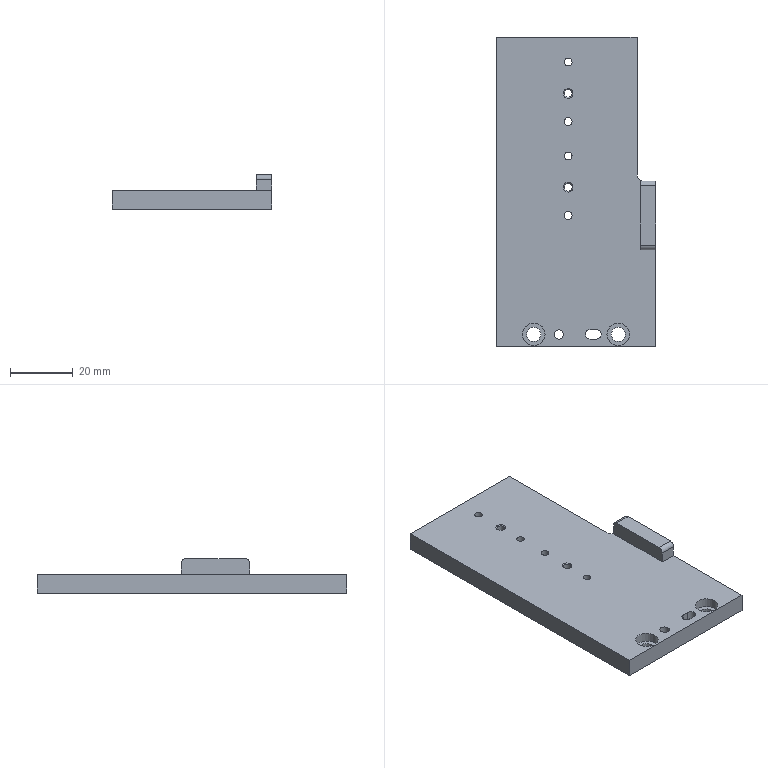Part | STEP file | ROTATION MC_NEW VER-0610_540 | 1 solid | 33 faces | box 51 x 99 x 11 mm | volume 28554 mm3 | cylinder 16 | plane 15 | cone 2 | commonest cylinder face diameters 3 x5 2.459 x4 2.5 x2 4.5 x2 7.2 x2 4 x1
STEP:
#1=CARTESIAN_POINT('',(217.301,684.268,-45.351));
#2=VERTEX_POINT('',#1);
#3=CARTESIAN_POINT('',(218.531,684.268,-45.351));
#4=DIRECTION('',(0.,0.,1.));
#5=DIRECTION('',(1.,0.,0.));
#6=AXIS2_PLACEMENT_3D('',#3,#4,#5);
#7=CIRCLE('',#6,1.23);
#8=EDGE_CURVE('',#2,#2,#7,.T.);
#9=ORIENTED_EDGE('',*,*,#8,.F.);
#10=CARTESIAN_POINT('',(217.301,684.268,-39.351));
#11=VERTEX_POINT('',#10);
#12=CARTESIAN_POINT('',(217.301,684.268,-151.257));
#13=DIRECTION('',(0.,0.,1.));
#14=VECTOR('',#13,1.23);
#15=LINE('',#12,#14);
#16=EDGE_CURVE('',#2,#11,#15,.T.);
#17=ORIENTED_EDGE('',*,*,#16,.T.);
#18=CARTESIAN_POINT('',(219.76,684.268,-39.351));
#19=VERTEX_POINT('',#18);
#20=CARTESIAN_POINT('',(218.531,684.268,-39.351));
#21=DIRECTION('',(0.,0.,-1.));
#22=DIRECTION('',(1.,0.,0.));
#23=AXIS2_PLACEMENT_3D('',#20,#21,#22);
#24=CIRCLE('',#23,1.23);
#25=EDGE_CURVE('',#19,#11,#24,.T.);
#26=ORIENTED_EDGE('',*,*,#25,.F.);
#27=CARTESIAN_POINT('',(218.531,684.268,-39.351));
#28=DIRECTION('',(0.,0.,-1.));
#29=DIRECTION('',(1.,0.,0.));
#30=AXIS2_PLACEMENT_3D('',#27,#28,#29);
#31=CIRCLE('',#30,1.23);
#32=EDGE_CURVE('',#11,#19,#31,.T.);
#33=ORIENTED_EDGE('',*,*,#32,.F.);
#34=ORIENTED_EDGE('',*,*,#16,.F.);
#35=EDGE_LOOP('',(#9,#17,#26,#33,#34));
#36=FACE_OUTER_BOUND('',#35,.T.);
#37=CARTESIAN_POINT('',(218.531,684.268,-151.257));
#38=DIRECTION('',(0.,0.,1.));
#39=DIRECTION('',(1.,0.,0.));
#40=AXIS2_PLACEMENT_3D('',#37,#38,#39);
#41=CYLINDRICAL_SURFACE('',#40,1.23);
#42=ADVANCED_FACE('',(#36),#41,.F.);
#43=CARTESIAN_POINT('',(217.301,703.268,-45.351));
#44=VERTEX_POINT('',#43);
#45=CARTESIAN_POINT('',(218.531,703.268,-45.351));
#46=DIRECTION('',(0.,0.,1.));
#47=DIRECTION('',(1.,0.,0.));
#48=AXIS2_PLACEMENT_3D('',#45,#46,#47);
#49=CIRCLE('',#48,1.23);
#50=EDGE_CURVE('',#44,#44,#49,.T.);
#51=ORIENTED_EDGE('',*,*,#50,.F.);
#52=CARTESIAN_POINT('',(217.301,703.268,-39.351));
#53=VERTEX_POINT('',#52);
#54=CARTESIAN_POINT('',(217.301,703.268,-151.257));
#55=DIRECTION('',(0.,0.,1.));
#56=VECTOR('',#55,1.23);
#57=LINE('',#54,#56);
#58=EDGE_CURVE('',#44,#53,#57,.T.);
#59=ORIENTED_EDGE('',*,*,#58,.T.);
#60=CARTESIAN_POINT('',(219.76,703.268,-39.351));
#61=VERTEX_POINT('',#60);
#62=CARTESIAN_POINT('',(218.531,703.268,-39.351));
#63=DIRECTION('',(0.,0.,-1.));
#64=DIRECTION('',(1.,0.,0.));
#65=AXIS2_PLACEMENT_3D('',#62,#63,#64);
#66=CIRCLE('',#65,1.23);
#67=EDGE_CURVE('',#61,#53,#66,.T.);
#68=ORIENTED_EDGE('',*,*,#67,.F.);
#69=CARTESIAN_POINT('',(218.531,703.268,-39.351));
#70=DIRECTION('',(0.,0.,-1.));
#71=DIRECTION('',(1.,0.,0.));
#72=AXIS2_PLACEMENT_3D('',#69,#70,#71);
#73=CIRCLE('',#72,1.23);
#74=EDGE_CURVE('',#53,#61,#73,.T.);
#75=ORIENTED_EDGE('',*,*,#74,.F.);
#76=ORIENTED_EDGE('',*,*,#58,.F.);
#77=EDGE_LOOP('',(#51,#59,#68,#75,#76));
#78=FACE_OUTER_BOUND('',#77,.T.);
#79=CARTESIAN_POINT('',(218.531,703.268,-151.257));
#80=DIRECTION('',(0.,0.,1.));
#81=DIRECTION('',(1.,0.,0.));
#82=AXIS2_PLACEMENT_3D('',#79,#80,#81);
#83=CYLINDRICAL_SURFACE('',#82,1.23);
#84=ADVANCED_FACE('',(#78),#83,.F.);
#85=CARTESIAN_POINT('',(217.301,673.268,-45.351));
#86=VERTEX_POINT('',#85);
#87=CARTESIAN_POINT('',(218.531,673.268,-45.351));
#88=DIRECTION('',(0.,0.,1.));
#89=DIRECTION('',(1.,0.,0.));
#90=AXIS2_PLACEMENT_3D('',#87,#88,#89);
#91=CIRCLE('',#90,1.23);
#92=EDGE_CURVE('',#86,#86,#91,.T.);
#93=ORIENTED_EDGE('',*,*,#92,.F.);
#94=CARTESIAN_POINT('',(217.301,673.268,-39.351));
#95=VERTEX_POINT('',#94);
#96=CARTESIAN_POINT('',(217.301,673.268,-151.257));
#97=DIRECTION('',(0.,0.,1.));
#98=VECTOR('',#97,1.23);
#99=LINE('',#96,#98);
#100=EDGE_CURVE('',#86,#95,#99,.T.);
#101=ORIENTED_EDGE('',*,*,#100,.T.);
#102=CARTESIAN_POINT('',(219.76,673.268,-39.351));
#103=VERTEX_POINT('',#102);
#104=CARTESIAN_POINT('',(218.531,673.268,-39.351));
#105=DIRECTION('',(0.,0.,-1.));
#106=DIRECTION('',(1.,0.,0.));
#107=AXIS2_PLACEMENT_3D('',#104,#105,#106);
#108=CIRCLE('',#107,1.23);
#109=EDGE_CURVE('',#103,#95,#108,.T.);
#110=ORIENTED_EDGE('',*,*,#109,.F.);
#111=CARTESIAN_POINT('',(218.531,673.268,-39.351));
#112=DIRECTION('',(0.,0.,-1.));
#113=DIRECTION('',(1.,0.,0.));
#114=AXIS2_PLACEMENT_3D('',#111,#112,#113);
#115=CIRCLE('',#114,1.23);
#116=EDGE_CURVE('',#95,#103,#115,.T.);
#117=ORIENTED_EDGE('',*,*,#116,.F.);
#118=ORIENTED_EDGE('',*,*,#100,.F.);
#119=EDGE_LOOP('',(#93,#101,#110,#117,#118));
#120=FACE_OUTER_BOUND('',#119,.T.);
#121=CARTESIAN_POINT('',(218.531,673.268,-151.257));
#122=DIRECTION('',(0.,0.,1.));
#123=DIRECTION('',(1.,0.,0.));
#124=AXIS2_PLACEMENT_3D('',#121,#122,#123);
#125=CYLINDRICAL_SURFACE('',#124,1.23);
#126=ADVANCED_FACE('',(#120),#125,.F.);
#127=CARTESIAN_POINT('',(217.301,654.268,-45.351));
#128=VERTEX_POINT('',#127);
#129=CARTESIAN_POINT('',(218.531,654.268,-45.351));
#130=DIRECTION('',(0.,0.,1.));
#131=DIRECTION('',(1.,0.,0.));
#132=AXIS2_PLACEMENT_3D('',#129,#130,#131);
#133=CIRCLE('',#132,1.23);
#134=EDGE_CURVE('',#128,#128,#133,.T.);
#135=ORIENTED_EDGE('',*,*,#134,.F.);
#136=CARTESIAN_POINT('',(217.301,654.268,-39.351));
#137=VERTEX_POINT('',#136);
#138=CARTESIAN_POINT('',(217.301,654.268,-151.257));
#139=DIRECTION('',(0.,0.,1.));
#140=VECTOR('',#139,1.23);
#141=LINE('',#138,#140);
#142=EDGE_CURVE('',#128,#137,#141,.T.);
#143=ORIENTED_EDGE('',*,*,#142,.T.);
#144=CARTESIAN_POINT('',(219.76,654.268,-39.351));
#145=VERTEX_POINT('',#144);
#146=CARTESIAN_POINT('',(218.531,654.268,-39.351));
#147=DIRECTION('',(0.,0.,-1.));
#148=DIRECTION('',(1.,0.,0.));
#149=AXIS2_PLACEMENT_3D('',#146,#147,#148);
#150=CIRCLE('',#149,1.23);
#151=EDGE_CURVE('',#145,#137,#150,.T.);
#152=ORIENTED_EDGE('',*,*,#151,.F.);
#153=CARTESIAN_POINT('',(218.531,654.268,-39.351));
#154=DIRECTION('',(0.,0.,-1.));
#155=DIRECTION('',(1.,0.,0.));
#156=AXIS2_PLACEMENT_3D('',#153,#154,#155);
#157=CIRCLE('',#156,1.23);
#158=EDGE_CURVE('',#137,#145,#157,.T.);
#159=ORIENTED_EDGE('',*,*,#158,.F.);
#160=ORIENTED_EDGE('',*,*,#142,.F.);
#161=EDGE_LOOP('',(#135,#143,#152,#159,#160));
#162=FACE_OUTER_BOUND('',#161,.T.);
#163=CARTESIAN_POINT('',(218.531,654.268,-151.257));
#164=DIRECTION('',(0.,0.,1.));
#165=DIRECTION('',(1.,0.,0.));
#166=AXIS2_PLACEMENT_3D('',#163,#164,#165);
#167=CYLINDRICAL_SURFACE('',#166,1.23);
#168=ADVANCED_FACE('',(#162),#167,.F.);
#169=CARTESIAN_POINT('',(240.531,711.268,-39.351));
#170=VERTEX_POINT('',#169);
#171=CARTESIAN_POINT('',(195.531,711.268,-39.351));
#172=VERTEX_POINT('',#171);
#173=CARTESIAN_POINT('',(216.167,711.268,-39.351));
#174=DIRECTION('',(-1.,0.,0.));
#175=VECTOR('',#174,10.);
#176=LINE('',#173,#175);
#177=EDGE_CURVE('',#170,#172,#176,.T.);
#178=ORIENTED_EDGE('',*,*,#177,.F.);
#179=CARTESIAN_POINT('',(240.531,711.268,-45.351));
#180=VERTEX_POINT('',#179);
#181=CARTESIAN_POINT('',(240.531,711.268,-45.351));
#182=DIRECTION('',(0.,0.,1.));
#183=VECTOR('',#182,9.5);
#184=LINE('',#181,#183);
#185=EDGE_CURVE('',#180,#170,#184,.T.);
#186=ORIENTED_EDGE('',*,*,#185,.F.);
#187=CARTESIAN_POINT('',(195.531,711.268,-45.351));
#188=VERTEX_POINT('',#187);
#189=CARTESIAN_POINT('',(240.531,711.268,-45.351));
#190=DIRECTION('',(-1.,0.,0.));
#191=VECTOR('',#190,45.);
#192=LINE('',#189,#191);
#193=EDGE_CURVE('',#180,#188,#192,.T.);
#194=ORIENTED_EDGE('',*,*,#193,.T.);
#195=CARTESIAN_POINT('',(195.531,711.268,-35.851));
#196=DIRECTION('',(0.,0.,-1.));
#197=VECTOR('',#196,9.5);
#198=LINE('',#195,#197);
#199=EDGE_CURVE('',#172,#188,#198,.T.);
#200=ORIENTED_EDGE('',*,*,#199,.F.);
#201=EDGE_LOOP('',(#178,#186,#194,#200));
#202=FACE_OUTER_BOUND('',#201,.T.);
#203=CARTESIAN_POINT('',(208.417,711.268,-65.091));
#204=DIRECTION('',(0.,1.,0.));
#205=DIRECTION('',(0.,0.,1.));
#206=AXIS2_PLACEMENT_3D('',#203,#204,#205);
#207=PLANE('',#206);
#208=ADVANCED_FACE('',(#202),#207,.T.);
#209=CARTESIAN_POINT('',(227.531,614.768,-39.351));
#210=VERTEX_POINT('',#209);
#211=CARTESIAN_POINT('',(227.531,617.768,-39.351));
#212=VERTEX_POINT('',#211);
#213=CARTESIAN_POINT('',(227.531,616.268,-39.351));
#214=DIRECTION('',(0.,0.,1.));
#215=DIRECTION('',(0.,-1.,0.));
#216=AXIS2_PLACEMENT_3D('',#213,#214,#215);
#217=CIRCLE('',#216,1.5);
#218=EDGE_CURVE('',#210,#212,#217,.T.);
#219=ORIENTED_EDGE('',*,*,#218,.T.);
#220=CARTESIAN_POINT('',(227.531,617.768,-45.351));
#221=VERTEX_POINT('',#220);
#222=CARTESIAN_POINT('',(227.531,617.768,-45.351));
#223=DIRECTION('',(0.,0.,1.));
#224=VECTOR('',#223,6.);
#225=LINE('',#222,#224);
#226=EDGE_CURVE('',#221,#212,#225,.T.);
#227=ORIENTED_EDGE('',*,*,#226,.F.);
#228=CARTESIAN_POINT('',(227.531,614.768,-45.351));
#229=VERTEX_POINT('',#228);
#230=CARTESIAN_POINT('',(227.531,616.268,-45.351));
#231=DIRECTION('',(0.,0.,-1.));
#232=DIRECTION('',(0.,1.,0.));
#233=AXIS2_PLACEMENT_3D('',#230,#231,#232);
#234=CIRCLE('',#233,1.5);
#235=EDGE_CURVE('',#221,#229,#234,.T.);
#236=ORIENTED_EDGE('',*,*,#235,.T.);
#237=CARTESIAN_POINT('',(227.531,614.768,-39.351));
#238=DIRECTION('',(0.,0.,-1.));
#239=VECTOR('',#238,6.);
#240=LINE('',#237,#239);
#241=EDGE_CURVE('',#210,#229,#240,.T.);
#242=ORIENTED_EDGE('',*,*,#241,.F.);
#243=EDGE_LOOP('',(#219,#227,#236,#242));
#244=FACE_OUTER_BOUND('',#243,.T.);
#245=CARTESIAN_POINT('',(227.531,616.268,-48.351));
#246=DIRECTION('',(0.,0.,1.));
#247=DIRECTION('',(1.,0.,0.));
#248=AXIS2_PLACEMENT_3D('',#245,#246,#247);
#249=CYLINDRICAL_SURFACE('',#248,1.5);
#250=ADVANCED_FACE('',(#244),#249,.F.);
#251=CARTESIAN_POINT('',(225.531,617.768,-39.351));
#252=VERTEX_POINT('',#251);
#253=CARTESIAN_POINT('',(225.531,614.768,-39.351));
#254=VERTEX_POINT('',#253);
#255=CARTESIAN_POINT('',(225.531,616.268,-39.351));
#256=DIRECTION('',(0.,0.,1.));
#257=DIRECTION('',(0.,-1.,0.));
#258=AXIS2_PLACEMENT_3D('',#255,#256,#257);
#259=CIRCLE('',#258,1.5);
#260=EDGE_CURVE('',#252,#254,#259,.T.);
#261=ORIENTED_EDGE('',*,*,#260,.T.);
#262=CARTESIAN_POINT('',(225.531,614.768,-45.351));
#263=VERTEX_POINT('',#262);
#264=CARTESIAN_POINT('',(225.531,614.768,-45.351));
#265=DIRECTION('',(0.,0.,1.));
#266=VECTOR('',#265,6.);
#267=LINE('',#264,#266);
#268=EDGE_CURVE('',#263,#254,#267,.T.);
#269=ORIENTED_EDGE('',*,*,#268,.F.);
#270=CARTESIAN_POINT('',(225.531,617.768,-45.351));
#271=VERTEX_POINT('',#270);
#272=CARTESIAN_POINT('',(225.531,616.268,-45.351));
#273=DIRECTION('',(0.,0.,-1.));
#274=DIRECTION('',(0.,1.,0.));
#275=AXIS2_PLACEMENT_3D('',#272,#273,#274);
#276=CIRCLE('',#275,1.5);
#277=EDGE_CURVE('',#263,#271,#276,.T.);
#278=ORIENTED_EDGE('',*,*,#277,.T.);
#279=CARTESIAN_POINT('',(225.531,617.768,-39.351));
#280=DIRECTION('',(0.,0.,-1.));
#281=VECTOR('',#280,6.);
#282=LINE('',#279,#281);
#283=EDGE_CURVE('',#252,#271,#282,.T.);
#284=ORIENTED_EDGE('',*,*,#283,.F.);
#285=EDGE_LOOP('',(#261,#269,#278,#284));
#286=FACE_OUTER_BOUND('',#285,.T.);
#287=CARTESIAN_POINT('',(225.531,616.268,-48.351));
#288=DIRECTION('',(0.,0.,1.));
#289=DIRECTION('',(-1.,0.,0.));
#290=AXIS2_PLACEMENT_3D('',#287,#288,#289);
#291=CYLINDRICAL_SURFACE('',#290,1.5);
#292=ADVANCED_FACE('',(#286),#291,.F.);
#293=CARTESIAN_POINT('',(227.531,617.768,-39.351));
#294=DIRECTION('',(-1.,0.,0.));
#295=VECTOR('',#294,2.);
#296=LINE('',#293,#295);
#297=EDGE_CURVE('',#212,#252,#296,.T.);
#298=ORIENTED_EDGE('',*,*,#297,.T.);
#299=ORIENTED_EDGE('',*,*,#283,.T.);
#300=CARTESIAN_POINT('',(225.531,617.768,-45.351));
#301=DIRECTION('',(1.,0.,0.));
#302=VECTOR('',#301,2.);
#303=LINE('',#300,#302);
#304=EDGE_CURVE('',#271,#221,#303,.T.);
#305=ORIENTED_EDGE('',*,*,#304,.T.);
#306=ORIENTED_EDGE('',*,*,#226,.T.);
#307=EDGE_LOOP('',(#298,#299,#305,#306));
#308=FACE_OUTER_BOUND('',#307,.T.);
#309=CARTESIAN_POINT('',(226.531,617.768,-48.351));
#310=DIRECTION('',(0.,1.,0.));
#311=DIRECTION('',(0.,0.,1.));
#312=AXIS2_PLACEMENT_3D('',#309,#310,#311);
#313=PLANE('',#312);
#314=ADVANCED_FACE('',(#308),#313,.F.);
#315=CARTESIAN_POINT('',(225.531,614.768,-39.351));
#316=DIRECTION('',(1.,0.,0.));
#317=VECTOR('',#316,2.);
#318=LINE('',#315,#317);
#319=EDGE_CURVE('',#254,#210,#318,.T.);
#320=ORIENTED_EDGE('',*,*,#319,.T.);
#321=ORIENTED_EDGE('',*,*,#241,.T.);
#322=CARTESIAN_POINT('',(227.531,614.768,-45.351));
#323=DIRECTION('',(-1.,0.,0.));
#324=VECTOR('',#323,2.);
#325=LINE('',#322,#324);
#326=EDGE_CURVE('',#229,#263,#325,.T.);
#327=ORIENTED_EDGE('',*,*,#326,.T.);
#328=ORIENTED_EDGE('',*,*,#268,.T.);
#329=EDGE_LOOP('',(#320,#321,#327,#328));
#330=FACE_OUTER_BOUND('',#329,.T.);
#331=CARTESIAN_POINT('',(226.531,614.768,-48.351));
#332=DIRECTION('',(0.,-1.,0.));
#333=DIRECTION('',(0.,0.,-1.));
#334=AXIS2_PLACEMENT_3D('',#331,#332,#333);
#335=PLANE('',#334);
#336=ADVANCED_FACE('',(#330),#335,.F.);
#337=CARTESIAN_POINT('',(246.531,612.268,-45.351));
#338=VERTEX_POINT('',#337);
#339=CARTESIAN_POINT('',(246.531,665.268,-45.351));
#340=VERTEX_POINT('',#339);
#341=CARTESIAN_POINT('',(246.531,612.268,-45.351));
#342=DIRECTION('',(0.,1.,0.));
#343=VECTOR('',#342,53.);
#344=LINE('',#341,#343);
#345=EDGE_CURVE('',#338,#340,#344,.T.);
#346=ORIENTED_EDGE('',*,*,#345,.F.);
#347=CARTESIAN_POINT('',(195.531,612.268,-45.351));
#348=VERTEX_POINT('',#347);
#349=CARTESIAN_POINT('',(195.531,612.268,-45.351));
#350=DIRECTION('',(1.,0.,0.));
#351=VECTOR('',#350,51.);
#352=LINE('',#349,#351);
#353=EDGE_CURVE('',#348,#338,#352,.T.);
#354=ORIENTED_EDGE('',*,*,#353,.F.);
#355=CARTESIAN_POINT('',(195.531,711.268,-45.351));
#356=DIRECTION('',(0.,-1.,0.));
#357=VECTOR('',#356,99.);
#358=LINE('',#355,#357);
#359=EDGE_CURVE('',#188,#348,#358,.T.);
#360=ORIENTED_EDGE('',*,*,#359,.F.);
#361=ORIENTED_EDGE('',*,*,#193,.F.);
#362=CARTESIAN_POINT('',(240.531,667.268,-45.351));
#363=VERTEX_POINT('',#362);
#364=CARTESIAN_POINT('',(240.531,667.268,-45.351));
#365=DIRECTION('',(0.,1.,0.));
#366=VECTOR('',#365,44.);
#367=LINE('',#364,#366);
#368=EDGE_CURVE('',#363,#180,#367,.T.);
#369=ORIENTED_EDGE('',*,*,#368,.F.);
#370=CARTESIAN_POINT('',(242.531,665.268,-45.351));
#371=VERTEX_POINT('',#370);
#372=CARTESIAN_POINT('',(242.531,667.268,-45.351));
#373=DIRECTION('',(0.,0.,-1.));
#374=DIRECTION('',(-0.7071,-0.7071,0.));
#375=AXIS2_PLACEMENT_3D('',#372,#373,#374);
#376=CIRCLE('',#375,2.);
#377=EDGE_CURVE('',#371,#363,#376,.T.);
#378=ORIENTED_EDGE('',*,*,#377,.F.);
#379=CARTESIAN_POINT('',(246.531,665.268,-45.351));
#380=DIRECTION('',(-1.,0.,0.));
#381=VECTOR('',#380,4.);
#382=LINE('',#379,#381);
#383=EDGE_CURVE('',#340,#371,#382,.T.);
#384=ORIENTED_EDGE('',*,*,#383,.F.);
#385=EDGE_LOOP('',(#346,#354,#360,#361,#369,#378,#384));
#386=FACE_OUTER_BOUND('',#385,.T.);
#387=ORIENTED_EDGE('',*,*,#8,.T.);
#388=EDGE_LOOP('',(#387));
#389=FACE_BOUND('',#388,.T.);
#390=ORIENTED_EDGE('',*,*,#50,.T.);
#391=EDGE_LOOP('',(#390));
#392=FACE_BOUND('',#391,.T.);
#393=ORIENTED_EDGE('',*,*,#92,.T.);
#394=EDGE_LOOP('',(#393));
#395=FACE_BOUND('',#394,.T.);
#396=ORIENTED_EDGE('',*,*,#134,.T.);
#397=EDGE_LOOP('',(#396));
#398=FACE_BOUND('',#397,.T.);
#399=CARTESIAN_POINT('',(209.781,616.268,-45.351));
#400=VERTEX_POINT('',#399);
#401=CARTESIAN_POINT('',(207.531,616.268,-45.351));
#402=DIRECTION('',(0.,0.,-1.));
#403=DIRECTION('',(1.,0.,0.));
#404=AXIS2_PLACEMENT_3D('',#401,#402,#403);
#405=CIRCLE('',#404,2.25);
#406=EDGE_CURVE('',#400,#400,#405,.T.);
#407=ORIENTED_EDGE('',*,*,#406,.F.);
#408=EDGE_LOOP('',(#407));
#409=FACE_BOUND('',#408,.T.);
#410=ORIENTED_EDGE('',*,*,#277,.F.);
#411=ORIENTED_EDGE('',*,*,#326,.F.);
#412=ORIENTED_EDGE('',*,*,#235,.F.);
#413=ORIENTED_EDGE('',*,*,#304,.F.);
#414=EDGE_LOOP('',(#410,#411,#412,#413));
#415=FACE_BOUND('',#414,.T.);
#416=CARTESIAN_POINT('',(218.531,694.518,-45.351));
#417=VERTEX_POINT('',#416);
#418=CARTESIAN_POINT('',(218.531,693.268,-45.351));
#419=DIRECTION('',(0.,0.,-1.));
#420=DIRECTION('',(0.,1.,0.));
#421=AXIS2_PLACEMENT_3D('',#418,#419,#420);
#422=CIRCLE('',#421,1.25);
#423=EDGE_CURVE('',#417,#417,#422,.T.);
#424=ORIENTED_EDGE('',*,*,#423,.F.);
#425=EDGE_LOOP('',(#424));
#426=FACE_BOUND('',#425,.T.);
#427=CARTESIAN_POINT('',(217.031,616.268,-45.351));
#428=VERTEX_POINT('',#427);
#429=CARTESIAN_POINT('',(215.531,616.268,-45.351));
#430=DIRECTION('',(0.,0.,-1.));
#431=DIRECTION('',(1.,0.,0.));
#432=AXIS2_PLACEMENT_3D('',#429,#430,#431);
#433=CIRCLE('',#432,1.5);
#434=EDGE_CURVE('',#428,#428,#433,.T.);
#435=ORIENTED_EDGE('',*,*,#434,.F.);
#436=EDGE_LOOP('',(#435));
#437=FACE_BOUND('',#436,.T.);
#438=CARTESIAN_POINT('',(236.781,616.268,-45.351));
#439=VERTEX_POINT('',#438);
#440=CARTESIAN_POINT('',(234.531,616.268,-45.351));
#441=DIRECTION('',(0.,0.,-1.));
#442=DIRECTION('',(1.,0.,0.));
#443=AXIS2_PLACEMENT_3D('',#440,#441,#442);
#444=CIRCLE('',#443,2.25);
#445=EDGE_CURVE('',#439,#439,#444,.T.);
#446=ORIENTED_EDGE('',*,*,#445,.F.);
#447=EDGE_LOOP('',(#446));
#448=FACE_BOUND('',#447,.T.);
#449=CARTESIAN_POINT('',(218.531,664.518,-45.351));
#450=VERTEX_POINT('',#449);
#451=CARTESIAN_POINT('',(218.531,663.268,-45.351));
#452=DIRECTION('',(0.,0.,-1.));
#453=DIRECTION('',(0.,1.,0.));
#454=AXIS2_PLACEMENT_3D('',#451,#452,#453);
#455=CIRCLE('',#454,1.25);
#456=EDGE_CURVE('',#450,#450,#455,.T.);
#457=ORIENTED_EDGE('',*,*,#456,.F.);
#458=EDGE_LOOP('',(#457));
#459=FACE_BOUND('',#458,.T.);
#460=CARTESIAN_POINT('',(227.031,630.268,-45.351));
#461=DIRECTION('',(0.,0.,-1.));
#462=DIRECTION('',(-1.,0.,0.));
#463=AXIS2_PLACEMENT_3D('',#460,#461,#462);
#464=PLANE('',#463);
#465=ADVANCED_FACE('',(#386,#389,#392,#395,#398,#409,#415,#426,#437,#448,#459),#464,.T.);
#466=ORIENTED_EDGE('',*,*,#185,.T.);
#467=CARTESIAN_POINT('',(240.531,667.268,-39.351));
#468=VERTEX_POINT('',#467);
#469=CARTESIAN_POINT('',(240.531,667.268,-39.351));
#470=DIRECTION('',(0.,1.,0.));
#471=VECTOR('',#470,41.);
#472=LINE('',#469,#471);
#473=EDGE_CURVE('',#468,#170,#472,.T.);
#474=ORIENTED_EDGE('',*,*,#473,.F.);
#475=CARTESIAN_POINT('',(240.531,667.268,-45.351));
#476=DIRECTION('',(0.,0.,1.));
#477=VECTOR('',#476,6.);
#478=LINE('',#475,#477);
#479=EDGE_CURVE('',#363,#468,#478,.T.);
#480=ORIENTED_EDGE('',*,*,#479,.F.);
#481=ORIENTED_EDGE('',*,*,#368,.T.);
#482=EDGE_LOOP('',(#466,#474,#480,#481));
#483=FACE_OUTER_BOUND('',#482,.T.);
#484=CARTESIAN_POINT('',(240.531,707.268,-39.351));
#485=DIRECTION('',(1.,0.,0.));
#486=DIRECTION('',(0.,0.,-1.));
#487=AXIS2_PLACEMENT_3D('',#484,#485,#486);
#488=PLANE('',#487);
#489=ADVANCED_FACE('',(#483),#488,.T.);
#490=CARTESIAN_POINT('',(241.531,665.268,-35.851));
#491=VERTEX_POINT('',#490);
#492=CARTESIAN_POINT('',(241.531,663.768,-34.351));
#493=VERTEX_POINT('',#492);
#494=CARTESIAN_POINT('',(241.531,663.768,-35.851));
#495=DIRECTION('',(1.,0.,0.));
#496=DIRECTION('',(0.,0.7071,0.7071));
#497=AXIS2_PLACEMENT_3D('',#494,#495,#496);
#498=CIRCLE('',#497,1.5);
#499=EDGE_CURVE('',#491,#493,#498,.T.);
#500=ORIENTED_EDGE('',*,*,#499,.F.);
#501=CARTESIAN_POINT('',(241.531,665.268,-39.351));
#502=VERTEX_POINT('',#501);
#503=CARTESIAN_POINT('',(241.531,665.268,-39.351));
#504=DIRECTION('',(0.,0.,1.));
#505=VECTOR('',#504,3.5);
#506=LINE('',#503,#505);
#507=EDGE_CURVE('',#502,#491,#506,.T.);
#508=ORIENTED_EDGE('',*,*,#507,.F.);
#509=CARTESIAN_POINT('',(241.531,643.268,-39.351));
#510=VERTEX_POINT('',#509);
#511=CARTESIAN_POINT('',(241.531,643.268,-39.351));
#512=DIRECTION('',(0.,1.,0.));
#513=VECTOR('',#512,22.);
#514=LINE('',#511,#513);
#515=EDGE_CURVE('',#510,#502,#514,.T.);
#516=ORIENTED_EDGE('',*,*,#515,.F.);
#517=CARTESIAN_POINT('',(241.531,643.268,-35.851));
#518=VERTEX_POINT('',#517);
#519=CARTESIAN_POINT('',(241.531,643.268,-39.351));
#520=DIRECTION('',(0.,0.,1.));
#521=VECTOR('',#520,3.5);
#522=LINE('',#519,#521);
#523=EDGE_CURVE('',#510,#518,#522,.T.);
#524=ORIENTED_EDGE('',*,*,#523,.T.);
#525=CARTESIAN_POINT('',(241.531,644.768,-34.351));
#526=VERTEX_POINT('',#525);
#527=CARTESIAN_POINT('',(241.531,644.768,-35.851));
#528=DIRECTION('',(1.,0.,0.));
#529=DIRECTION('',(0.,-0.7071,0.7071));
#530=AXIS2_PLACEMENT_3D('',#527,#528,#529);
#531=CIRCLE('',#530,1.5);
#532=EDGE_CURVE('',#526,#518,#531,.T.);
#533=ORIENTED_EDGE('',*,*,#532,.F.);
#534=CARTESIAN_POINT('',(241.531,644.768,-34.351));
#535=DIRECTION('',(0.,1.,0.));
#536=VECTOR('',#535,19.);
#537=LINE('',#534,#536);
#538=EDGE_CURVE('',#526,#493,#537,.T.);
#539=ORIENTED_EDGE('',*,*,#538,.T.);
#540=EDGE_LOOP('',(#500,#508,#516,#524,#533,#539));
#541=FACE_OUTER_BOUND('',#540,.T.);
#542=CARTESIAN_POINT('',(241.531,707.268,-39.351));
#543=DIRECTION('',(1.,0.,0.));
#544=DIRECTION('',(0.,0.,-1.));
#545=AXIS2_PLACEMENT_3D('',#542,#543,#544);
#546=PLANE('',#545);
#547=ADVANCED_FACE('',(#541),#546,.F.);
#548=CARTESIAN_POINT('',(246.531,643.268,-35.851));
#549=VERTEX_POINT('',#548);
#550=CARTESIAN_POINT('',(246.531,644.768,-34.351));
#551=VERTEX_POINT('',#550);
#552=CARTESIAN_POINT('',(246.531,644.768,-35.851));
#553=DIRECTION('',(-1.,0.,0.));
#554=DIRECTION('',(0.,-0.7071,0.7071));
#555=AXIS2_PLACEMENT_3D('',#552,#553,#554);
#556=CIRCLE('',#555,1.5);
#557=EDGE_CURVE('',#549,#551,#556,.T.);
#558=ORIENTED_EDGE('',*,*,#557,.T.);
#559=CARTESIAN_POINT('',(246.531,644.768,-34.351));
#560=DIRECTION('',(-1.,0.,0.));
#561=VECTOR('',#560,5.);
#562=LINE('',#559,#561);
#563=EDGE_CURVE('',#551,#526,#562,.T.);
#564=ORIENTED_EDGE('',*,*,#563,.T.);
#565=ORIENTED_EDGE('',*,*,#532,.T.);
#566=CARTESIAN_POINT('',(241.531,643.268,-35.851));
#567=DIRECTION('',(1.,0.,0.));
#568=VECTOR('',#567,5.);
#569=LINE('',#566,#568);
#570=EDGE_CURVE('',#518,#549,#569,.T.);
#571=ORIENTED_EDGE('',*,*,#570,.T.);
#572=EDGE_LOOP('',(#558,#564,#565,#571));
#573=FACE_OUTER_BOUND('',#572,.T.);
#574=CARTESIAN_POINT('',(221.224,644.768,-35.851));
#575=DIRECTION('',(-1.,0.,0.));
#576=DIRECTION('',(0.,-0.7071,0.7071));
#577=AXIS2_PLACEMENT_3D('',#574,#575,#576);
#578=CYLINDRICAL_SURFACE('',#577,1.5);
#579=ADVANCED_FACE('',(#573),#578,.T.);
#580=ORIENTED_EDGE('',*,*,#434,.T.);
#581=CARTESIAN_POINT('',(217.031,616.268,-39.351));
#582=VERTEX_POINT('',#581);
#583=CARTESIAN_POINT('',(217.031,616.268,-45.091));
#584=DIRECTION('',(0.,0.,1.));
#585=VECTOR('',#584,1.5);
#586=LINE('',#583,#585);
#587=EDGE_CURVE('',#428,#582,#586,.T.);
#588=ORIENTED_EDGE('',*,*,#587,.T.);
#589=CARTESIAN_POINT('',(215.531,616.268,-39.351));
#590=DIRECTION('',(0.,0.,1.));
#591=DIRECTION('',(1.,0.,0.));
#592=AXIS2_PLACEMENT_3D('',#589,#590,#591);
#593=CIRCLE('',#592,1.5);
#594=EDGE_CURVE('',#582,#582,#593,.T.);
#595=ORIENTED_EDGE('',*,*,#594,.T.);
#596=ORIENTED_EDGE('',*,*,#587,.F.);
#597=EDGE_LOOP('',(#580,#588,#595,#596));
#598=FACE_OUTER_BOUND('',#597,.T.);
#599=CARTESIAN_POINT('',(215.531,616.268,-45.091));
#600=DIRECTION('',(0.,0.,1.));
#601=DIRECTION('',(-1.,0.,0.));
#602=AXIS2_PLACEMENT_3D('',#599,#600,#601);
#603=CYLINDRICAL_SURFACE('',#602,1.5);
#604=ADVANCED_FACE('',(#598),#603,.F.);
#605=CARTESIAN_POINT('',(218.531,662.018,-39.651));
#606=VERTEX_POINT('',#605);
#607=CARTESIAN_POINT('',(218.531,664.518,-39.651));
#608=VERTEX_POINT('',#607);
#609=CARTESIAN_POINT('',(218.531,663.268,-39.651));
#610=DIRECTION('',(0.,0.,-1.));
#611=DIRECTION('',(0.,-1.,0.));
#612=AXIS2_PLACEMENT_3D('',#609,#610,#611);
#613=CIRCLE('',#612,1.25);
#614=EDGE_CURVE('',#606,#608,#613,.T.);
#615=ORIENTED_EDGE('',*,*,#614,.F.);
#616=CARTESIAN_POINT('',(218.531,663.268,-39.651));
#617=DIRECTION('',(0.,0.,-1.));
#618=DIRECTION('',(0.,-1.,0.));
#619=AXIS2_PLACEMENT_3D('',#616,#617,#618);
#620=CIRCLE('',#619,1.25);
#621=EDGE_CURVE('',#608,#606,#620,.T.);
#622=ORIENTED_EDGE('',*,*,#621,.F.);
#623=CARTESIAN_POINT('',(218.531,664.518,-22.351));
#624=DIRECTION('',(0.,0.,-1.));
#625=VECTOR('',#624,1.25);
#626=LINE('',#623,#625);
#627=EDGE_CURVE('',#608,#450,#626,.T.);
#628=ORIENTED_EDGE('',*,*,#627,.T.);
#629=ORIENTED_EDGE('',*,*,#456,.T.);
#630=ORIENTED_EDGE('',*,*,#627,.F.);
#631=EDGE_LOOP('',(#615,#622,#628,#629,#630));
#632=FACE_OUTER_BOUND('',#631,.T.);
#633=CARTESIAN_POINT('',(218.531,663.268,-22.351));
#634=DIRECTION('',(0.,0.,-1.));
#635=DIRECTION('',(0.,-1.,0.));
#636=AXIS2_PLACEMENT_3D('',#633,#634,#635);
#637=CYLINDRICAL_SURFACE('',#636,1.25);
#638=ADVANCED_FACE('',(#632),#637,.F.);
#639=CARTESIAN_POINT('',(246.531,663.768,-34.351));
#640=VERTEX_POINT('',#639);
#641=CARTESIAN_POINT('',(246.531,665.268,-35.851));
#642=VERTEX_POINT('',#641);
#643=CARTESIAN_POINT('',(246.531,663.768,-35.851));
#644=DIRECTION('',(-1.,0.,0.));
#645=DIRECTION('',(0.,0.7071,0.7071));
#646=AXIS2_PLACEMENT_3D('',#643,#644,#645);
#647=CIRCLE('',#646,1.5);
#648=EDGE_CURVE('',#640,#642,#647,.T.);
#649=ORIENTED_EDGE('',*,*,#648,.T.);
#650=CARTESIAN_POINT('',(246.531,665.268,-35.851));
#651=DIRECTION('',(-1.,0.,0.));
#652=VECTOR('',#651,5.);
#653=LINE('',#650,#652);
#654=EDGE_CURVE('',#642,#491,#653,.T.);
#655=ORIENTED_EDGE('',*,*,#654,.T.);
#656=ORIENTED_EDGE('',*,*,#499,.T.);
#657=CARTESIAN_POINT('',(241.531,663.768,-34.351));
#658=DIRECTION('',(1.,0.,0.));
#659=VECTOR('',#658,5.);
#660=LINE('',#657,#659);
#661=EDGE_CURVE('',#493,#640,#660,.T.);
#662=ORIENTED_EDGE('',*,*,#661,.T.);
#663=EDGE_LOOP('',(#649,#655,#656,#662));
#664=FACE_OUTER_BOUND('',#663,.T.);
#665=CARTESIAN_POINT('',(233.974,663.768,-35.851));
#666=DIRECTION('',(-1.,0.,0.));
#667=DIRECTION('',(0.,0.7071,0.7071));
#668=AXIS2_PLACEMENT_3D('',#665,#666,#667);
#669=CYLINDRICAL_SURFACE('',#668,1.5);
#670=ADVANCED_FACE('',(#664),#669,.T.);
#671=CARTESIAN_POINT('',(238.131,616.268,-42.351));
#672=VERTEX_POINT('',#671);
#673=CARTESIAN_POINT('',(234.531,616.268,-42.351));
#674=DIRECTION('',(0.,0.,1.));
#675=DIRECTION('',(1.,0.,0.));
#676=AXIS2_PLACEMENT_3D('',#673,#674,#675);
#677=CIRCLE('',#676,3.6);
#678=EDGE_CURVE('',#672,#672,#677,.T.);
#679=ORIENTED_EDGE('',*,*,#678,.T.);
#680=EDGE_LOOP('',(#679));
#681=FACE_OUTER_BOUND('',#680,.T.);
#682=CARTESIAN_POINT('',(236.781,616.268,-42.351));
#683=VERTEX_POINT('',#682);
#684=CARTESIAN_POINT('',(234.531,616.268,-42.351));
#685=DIRECTION('',(0.,0.,-1.));
#686=DIRECTION('',(1.,0.,0.));
#687=AXIS2_PLACEMENT_3D('',#684,#685,#686);
#688=CIRCLE('',#687,2.25);
#689=EDGE_CURVE('',#683,#683,#688,.T.);
#690=ORIENTED_EDGE('',*,*,#689,.T.);
#691=EDGE_LOOP('',(#690));
#692=FACE_BOUND('',#691,.T.);
#693=CARTESIAN_POINT('',(232.261,632.268,-42.351));
#694=DIRECTION('',(0.,0.,1.));
#695=DIRECTION('',(1.,0.,0.));
#696=AXIS2_PLACEMENT_3D('',#693,#694,#695);
#697=PLANE('',#696);
#698=ADVANCED_FACE('',(#681,#692),#697,.T.);
#699=CARTESIAN_POINT('',(242.531,665.268,-39.351));
#700=VERTEX_POINT('',#699);
#701=CARTESIAN_POINT('',(242.531,667.268,-39.351));
#702=DIRECTION('',(0.,0.,-1.));
#703=DIRECTION('',(-0.7071,-0.7071,0.));
#704=AXIS2_PLACEMENT_3D('',#701,#702,#703);
#705=CIRCLE('',#704,2.);
#706=EDGE_CURVE('',#700,#468,#705,.T.);
#707=ORIENTED_EDGE('',*,*,#706,.F.);
#708=CARTESIAN_POINT('',(242.531,665.268,-39.351));
#709=DIRECTION('',(0.,0.,-1.));
#710=VECTOR('',#709,6.);
#711=LINE('',#708,#710);
#712=EDGE_CURVE('',#700,#371,#711,.T.);
#713=ORIENTED_EDGE('',*,*,#712,.T.);
#714=ORIENTED_EDGE('',*,*,#377,.T.);
#715=ORIENTED_EDGE('',*,*,#479,.T.);
#716=EDGE_LOOP('',(#707,#713,#714,#715));
#717=FACE_OUTER_BOUND('',#716,.T.);
#718=CARTESIAN_POINT('',(242.531,667.268,-36.851));
#719=DIRECTION('',(0.,0.,-1.));
#720=DIRECTION('',(-0.7071,-0.7071,0.));
#721=AXIS2_PLACEMENT_3D('',#718,#719,#720);
#722=CYLINDRICAL_SURFACE('',#721,2.);
#723=ADVANCED_FACE('',(#717),#722,.F.);
#724=ORIENTED_EDGE('',*,*,#177,.T.);
#725=CARTESIAN_POINT('',(195.531,612.268,-39.351));
#726=VERTEX_POINT('',#725);
#727=CARTESIAN_POINT('',(195.531,612.268,-39.351));
#728=DIRECTION('',(0.,1.,0.));
#729=VECTOR('',#728,96.);
#730=LINE('',#727,#729);
#731=EDGE_CURVE('',#726,#172,#730,.T.);
#732=ORIENTED_EDGE('',*,*,#731,.F.);
#733=CARTESIAN_POINT('',(246.531,612.268,-39.351));
#734=VERTEX_POINT('',#733);
#735=CARTESIAN_POINT('',(195.531,612.268,-39.351));
#736=DIRECTION('',(1.,0.,0.));
#737=VECTOR('',#736,51.);
#738=LINE('',#735,#737);
#739=EDGE_CURVE('',#726,#734,#738,.T.);
#740=ORIENTED_EDGE('',*,*,#739,.T.);
#741=CARTESIAN_POINT('',(246.531,643.268,-39.351));
#742=VERTEX_POINT('',#741);
#743=CARTESIAN_POINT('',(246.531,612.268,-39.351));
#744=DIRECTION('',(0.,1.,0.));
#745=VECTOR('',#744,31.);
#746=LINE('',#743,#745);
#747=EDGE_CURVE('',#734,#742,#746,.T.);
#748=ORIENTED_EDGE('',*,*,#747,.T.);
#749=CARTESIAN_POINT('',(241.531,643.268,-39.351));
#750=DIRECTION('',(1.,0.,0.));
#751=VECTOR('',#750,5.);
#752=LINE('',#749,#751);
#753=EDGE_CURVE('',#510,#742,#752,.T.);
#754=ORIENTED_EDGE('',*,*,#753,.F.);
#755=ORIENTED_EDGE('',*,*,#515,.T.);
#756=CARTESIAN_POINT('',(242.531,665.268,-39.351));
#757=DIRECTION('',(-1.,0.,0.));
#758=VECTOR('',#757,1.);
#759=LINE('',#756,#758);
#760=EDGE_CURVE('',#700,#502,#759,.T.);
#761=ORIENTED_EDGE('',*,*,#760,.F.);
#762=ORIENTED_EDGE('',*,*,#706,.T.);
#763=ORIENTED_EDGE('',*,*,#473,.T.);
#764=EDGE_LOOP('',(#724,#732,#740,#748,#754,#755,#761,#762,#763));
#765=FACE_OUTER_BOUND('',#764,.T.);
#766=ORIENTED_EDGE('',*,*,#25,.T.);
#767=ORIENTED_EDGE('',*,*,#32,.T.);
#768=EDGE_LOOP('',(#766,#767));
#769=FACE_BOUND('',#768,.T.);
#770=ORIENTED_EDGE('',*,*,#67,.T.);
#771=ORIENTED_EDGE('',*,*,#74,.T.);
#772=EDGE_LOOP('',(#770,#771));
#773=FACE_BOUND('',#772,.T.);
#774=ORIENTED_EDGE('',*,*,#109,.T.);
#775=ORIENTED_EDGE('',*,*,#116,.T.);
#776=EDGE_LOOP('',(#774,#775));
#777=FACE_BOUND('',#776,.T.);
#778=ORIENTED_EDGE('',*,*,#151,.T.);
#779=ORIENTED_EDGE('',*,*,#158,.T.);
#780=EDGE_LOOP('',(#778,#779));
#781=FACE_BOUND('',#780,.T.);
#782=CARTESIAN_POINT('',(218.531,661.718,-39.351));
#783=VERTEX_POINT('',#782);
#784=CARTESIAN_POINT('',(218.531,663.268,-39.351));
#785=DIRECTION('',(0.,0.,1.));
#786=DIRECTION('',(0.,-1.,0.));
#787=AXIS2_PLACEMENT_3D('',#784,#785,#786);
#788=CIRCLE('',#787,1.55);
#789=EDGE_CURVE('',#783,#783,#788,.T.);
#790=ORIENTED_EDGE('',*,*,#789,.F.);
#791=EDGE_LOOP('',(#790));
#792=FACE_BOUND('',#791,.T.);
#793=ORIENTED_EDGE('',*,*,#260,.F.);
#794=ORIENTED_EDGE('',*,*,#297,.F.);
#795=ORIENTED_EDGE('',*,*,#218,.F.);
#796=ORIENTED_EDGE('',*,*,#319,.F.);
#797=EDGE_LOOP('',(#793,#794,#795,#796));
#798=FACE_BOUND('',#797,.T.);
#799=CARTESIAN_POINT('',(238.131,616.268,-39.351));
#800=VERTEX_POINT('',#799);
#801=CARTESIAN_POINT('',(234.531,616.268,-39.351));
#802=DIRECTION('',(0.,0.,-1.));
#803=DIRECTION('',(1.,0.,0.));
#804=AXIS2_PLACEMENT_3D('',#801,#802,#803);
#805=CIRCLE('',#804,3.6);
#806=EDGE_CURVE('',#800,#800,#805,.T.);
#807=ORIENTED_EDGE('',*,*,#806,.T.);
#808=EDGE_LOOP('',(#807));
#809=FACE_BOUND('',#808,.T.);
#810=ORIENTED_EDGE('',*,*,#594,.F.);
#811=EDGE_LOOP('',(#810));
#812=FACE_BOUND('',#811,.T.);
#813=CARTESIAN_POINT('',(211.131,616.268,-39.351));
#814=VERTEX_POINT('',#813);
#815=CARTESIAN_POINT('',(207.531,616.268,-39.351));
#816=DIRECTION('',(0.,0.,1.));
#817=DIRECTION('',(1.,0.,0.));
#818=AXIS2_PLACEMENT_3D('',#815,#816,#817);
#819=CIRCLE('',#818,3.6);
#820=EDGE_CURVE('',#814,#814,#819,.T.);
#821=ORIENTED_EDGE('',*,*,#820,.F.);
#822=EDGE_LOOP('',(#821));
#823=FACE_BOUND('',#822,.T.);
#824=CARTESIAN_POINT('',(218.531,691.718,-39.351));
#825=VERTEX_POINT('',#824);
#826=CARTESIAN_POINT('',(218.531,693.268,-39.351));
#827=DIRECTION('',(0.,0.,1.));
#828=DIRECTION('',(0.,-1.,0.));
#829=AXIS2_PLACEMENT_3D('',#826,#827,#828);
#830=CIRCLE('',#829,1.55);
#831=EDGE_CURVE('',#825,#825,#830,.T.);
#832=ORIENTED_EDGE('',*,*,#831,.F.);
#833=EDGE_LOOP('',(#832));
#834=FACE_BOUND('',#833,.T.);
#835=CARTESIAN_POINT('',(223.917,622.268,-39.351));
#836=DIRECTION('',(0.,0.,1.));
#837=DIRECTION('',(1.,0.,0.));
#838=AXIS2_PLACEMENT_3D('',#835,#836,#837);
#839=PLANE('',#838);
#840=ADVANCED_FACE('',(#765,#769,#773,#777,#781,#792,#798,#809,#812,#823,#834),#839,.T.);
#841=CARTESIAN_POINT('',(246.531,612.268,-39.351));
#842=DIRECTION('',(0.,0.,-1.));
#843=VECTOR('',#842,6.);
#844=LINE('',#841,#843);
#845=EDGE_CURVE('',#734,#338,#844,.T.);
#846=ORIENTED_EDGE('',*,*,#845,.F.);
#847=ORIENTED_EDGE('',*,*,#739,.F.);
#848=CARTESIAN_POINT('',(195.531,612.268,-45.351));
#849=DIRECTION('',(0.,0.,1.));
#850=VECTOR('',#849,6.);
#851=LINE('',#848,#850);
#852=EDGE_CURVE('',#348,#726,#851,.T.);
#853=ORIENTED_EDGE('',*,*,#852,.F.);
#854=ORIENTED_EDGE('',*,*,#353,.T.);
#855=EDGE_LOOP('',(#846,#847,#853,#854));
#856=FACE_OUTER_BOUND('',#855,.T.);
#857=CARTESIAN_POINT('',(208.417,612.268,-65.091));
#858=DIRECTION('',(0.,1.,0.));
#859=DIRECTION('',(0.,0.,1.));
#860=AXIS2_PLACEMENT_3D('',#857,#858,#859);
#861=PLANE('',#860);
#862=ADVANCED_FACE('',(#856),#861,.F.);
#863=ORIENTED_EDGE('',*,*,#712,.F.);
#864=ORIENTED_EDGE('',*,*,#760,.T.);
#865=ORIENTED_EDGE('',*,*,#507,.T.);
#866=ORIENTED_EDGE('',*,*,#654,.F.);
#867=CARTESIAN_POINT('',(246.531,665.268,-45.351));
#868=DIRECTION('',(0.,0.,1.));
#869=VECTOR('',#868,9.5);
#870=LINE('',#867,#869);
#871=EDGE_CURVE('',#340,#642,#870,.T.);
#872=ORIENTED_EDGE('',*,*,#871,.F.);
#873=ORIENTED_EDGE('',*,*,#383,.T.);
#874=EDGE_LOOP('',(#863,#864,#865,#866,#872,#873));
#875=FACE_OUTER_BOUND('',#874,.T.);
#876=CARTESIAN_POINT('',(244.031,665.268,-34.351));
#877=DIRECTION('',(0.,1.,0.));
#878=DIRECTION('',(0.,0.,1.));
#879=AXIS2_PLACEMENT_3D('',#876,#877,#878);
#880=PLANE('',#879);
#881=ADVANCED_FACE('',(#875),#880,.T.);
#882=ORIENTED_EDGE('',*,*,#570,.F.);
#883=ORIENTED_EDGE('',*,*,#523,.F.);
#884=ORIENTED_EDGE('',*,*,#753,.T.);
#885=CARTESIAN_POINT('',(246.531,643.268,-35.851));
#886=DIRECTION('',(0.,0.,-1.));
#887=VECTOR('',#886,3.5);
#888=LINE('',#885,#887);
#889=EDGE_CURVE('',#549,#742,#888,.T.);
#890=ORIENTED_EDGE('',*,*,#889,.F.);
#891=EDGE_LOOP('',(#882,#883,#884,#890));
#892=FACE_OUTER_BOUND('',#891,.T.);
#893=CARTESIAN_POINT('',(218.531,643.268,-32.351));
#894=DIRECTION('',(0.,-1.,0.));
#895=DIRECTION('',(0.,0.,-1.));
#896=AXIS2_PLACEMENT_3D('',#893,#894,#895);
#897=PLANE('',#896);
#898=ADVANCED_FACE('',(#892),#897,.T.);
#899=CARTESIAN_POINT('',(211.131,616.268,-42.351));
#900=VERTEX_POINT('',#899);
#901=CARTESIAN_POINT('',(207.531,616.268,-42.351));
#902=DIRECTION('',(0.,0.,1.));
#903=DIRECTION('',(1.,0.,0.));
#904=AXIS2_PLACEMENT_3D('',#901,#902,#903);
#905=CIRCLE('',#904,3.6);
#906=EDGE_CURVE('',#900,#900,#905,.T.);
#907=ORIENTED_EDGE('',*,*,#906,.F.);
#908=CARTESIAN_POINT('',(211.131,616.268,-45.091));
#909=DIRECTION('',(0.,0.,1.));
#910=VECTOR('',#909,3.6);
#911=LINE('',#908,#910);
#912=EDGE_CURVE('',#900,#814,#911,.T.);
#913=ORIENTED_EDGE('',*,*,#912,.T.);
#914=ORIENTED_EDGE('',*,*,#820,.T.);
#915=ORIENTED_EDGE('',*,*,#912,.F.);
#916=EDGE_LOOP('',(#907,#913,#914,#915));
#917=FACE_OUTER_BOUND('',#916,.T.);
#918=CARTESIAN_POINT('',(207.531,616.268,-45.091));
#919=DIRECTION('',(0.,0.,1.));
#920=DIRECTION('',(-1.,0.,0.));
#921=AXIS2_PLACEMENT_3D('',#918,#919,#920);
#922=CYLINDRICAL_SURFACE('',#921,3.6);
#923=ADVANCED_FACE('',(#917),#922,.F.);
#924=CARTESIAN_POINT('',(218.531,692.018,-39.651));
#925=VERTEX_POINT('',#924);
#926=CARTESIAN_POINT('',(218.531,694.518,-39.651));
#927=VERTEX_POINT('',#926);
#928=CARTESIAN_POINT('',(218.531,693.268,-39.651));
#929=DIRECTION('',(0.,0.,-1.));
#930=DIRECTION('',(0.,-1.,0.));
#931=AXIS2_PLACEMENT_3D('',#928,#929,#930);
#932=CIRCLE('',#931,1.25);
#933=EDGE_CURVE('',#925,#927,#932,.T.);
#934=ORIENTED_EDGE('',*,*,#933,.F.);
#935=CARTESIAN_POINT('',(218.531,693.268,-39.651));
#936=DIRECTION('',(0.,0.,-1.));
#937=DIRECTION('',(0.,-1.,0.));
#938=AXIS2_PLACEMENT_3D('',#935,#936,#937);
#939=CIRCLE('',#938,1.25);
#940=EDGE_CURVE('',#927,#925,#939,.T.);
#941=ORIENTED_EDGE('',*,*,#940,.F.);
#942=CARTESIAN_POINT('',(218.531,694.518,-22.351));
#943=DIRECTION('',(0.,0.,-1.));
#944=VECTOR('',#943,1.25);
#945=LINE('',#942,#944);
#946=EDGE_CURVE('',#927,#417,#945,.T.);
#947=ORIENTED_EDGE('',*,*,#946,.T.);
#948=ORIENTED_EDGE('',*,*,#423,.T.);
#949=ORIENTED_EDGE('',*,*,#946,.F.);
#950=EDGE_LOOP('',(#934,#941,#947,#948,#949));
#951=FACE_OUTER_BOUND('',#950,.T.);
#952=CARTESIAN_POINT('',(218.531,693.268,-22.351));
#953=DIRECTION('',(0.,0.,-1.));
#954=DIRECTION('',(0.,-1.,0.));
#955=AXIS2_PLACEMENT_3D('',#952,#953,#954);
#956=CYLINDRICAL_SURFACE('',#955,1.25);
#957=ADVANCED_FACE('',(#951),#956,.F.);
#958=ORIENTED_EDGE('',*,*,#731,.T.);
#959=ORIENTED_EDGE('',*,*,#199,.T.);
#960=ORIENTED_EDGE('',*,*,#359,.T.);
#961=ORIENTED_EDGE('',*,*,#852,.T.);
#962=EDGE_LOOP('',(#958,#959,#960,#961));
#963=FACE_OUTER_BOUND('',#962,.T.);
#964=CARTESIAN_POINT('',(195.531,622.268,-91.091));
#965=DIRECTION('',(-1.,0.,0.));
#966=DIRECTION('',(0.,0.,1.));
#967=AXIS2_PLACEMENT_3D('',#964,#965,#966);
#968=PLANE('',#967);
#969=ADVANCED_FACE('',(#963),#968,.T.);
#970=ORIENTED_EDGE('',*,*,#445,.T.);
#971=CARTESIAN_POINT('',(236.781,616.268,-48.091));
#972=DIRECTION('',(0.,0.,1.));
#973=VECTOR('',#972,2.25);
#974=LINE('',#971,#973);
#975=EDGE_CURVE('',#439,#683,#974,.T.);
#976=ORIENTED_EDGE('',*,*,#975,.T.);
#977=ORIENTED_EDGE('',*,*,#689,.F.);
#978=ORIENTED_EDGE('',*,*,#975,.F.);
#979=EDGE_LOOP('',(#970,#976,#977,#978));
#980=FACE_OUTER_BOUND('',#979,.T.);
#981=CARTESIAN_POINT('',(234.531,616.268,-48.091));
#982=DIRECTION('',(0.,0.,1.));
#983=DIRECTION('',(-1.,0.,0.));
#984=AXIS2_PLACEMENT_3D('',#981,#982,#983);
#985=CYLINDRICAL_SURFACE('',#984,2.25);
#986=ADVANCED_FACE('',(#980),#985,.F.);
#987=ORIENTED_EDGE('',*,*,#614,.T.);
#988=ORIENTED_EDGE('',*,*,#621,.T.);
#989=CARTESIAN_POINT('',(218.531,661.718,-39.351));
#990=DIRECTION('',(0.,-0.7071,0.7071));
#991=VECTOR('',#990,1.55);
#992=LINE('',#989,#991);
#993=EDGE_CURVE('',#606,#783,#992,.T.);
#994=ORIENTED_EDGE('',*,*,#993,.T.);
#995=ORIENTED_EDGE('',*,*,#789,.T.);
#996=ORIENTED_EDGE('',*,*,#993,.F.);
#997=EDGE_LOOP('',(#987,#988,#994,#995,#996));
#998=FACE_OUTER_BOUND('',#997,.T.);
#999=CARTESIAN_POINT('',(218.531,663.268,-39.351));
#1000=DIRECTION('',(0.,0.,1.));
#1001=DIRECTION('',(0.,1.,0.));
#1002=AXIS2_PLACEMENT_3D('',#999,#1000,#1001);
#1003=CONICAL_SURFACE('',#1002,1.55,0.7854);
#1004=ADVANCED_FACE('',(#998),#1003,.F.);
#1005=ORIENTED_EDGE('',*,*,#661,.F.);
#1006=ORIENTED_EDGE('',*,*,#538,.F.);
#1007=ORIENTED_EDGE('',*,*,#563,.F.);
#1008=CARTESIAN_POINT('',(246.531,644.768,-34.351));
#1009=DIRECTION('',(0.,1.,0.));
#1010=VECTOR('',#1009,19.);
#1011=LINE('',#1008,#1010);
#1012=EDGE_CURVE('',#551,#640,#1011,.T.);
#1013=ORIENTED_EDGE('',*,*,#1012,.T.);
#1014=EDGE_LOOP('',(#1005,#1006,#1007,#1013));
#1015=FACE_OUTER_BOUND('',#1014,.T.);
#1016=CARTESIAN_POINT('',(223.917,622.268,-34.351));
#1017=DIRECTION('',(0.,0.,1.));
#1018=DIRECTION('',(1.,0.,0.));
#1019=AXIS2_PLACEMENT_3D('',#1016,#1017,#1018);
#1020=PLANE('',#1019);
#1021=ADVANCED_FACE('',(#1015),#1020,.T.);
#1022=ORIENTED_EDGE('',*,*,#406,.T.);
#1023=CARTESIAN_POINT('',(209.781,616.268,-42.351));
#1024=VERTEX_POINT('',#1023);
#1025=CARTESIAN_POINT('',(209.781,616.268,-48.091));
#1026=DIRECTION('',(0.,0.,1.));
#1027=VECTOR('',#1026,2.25);
#1028=LINE('',#1025,#1027);
#1029=EDGE_CURVE('',#400,#1024,#1028,.T.);
#1030=ORIENTED_EDGE('',*,*,#1029,.T.);
#1031=CARTESIAN_POINT('',(207.531,616.268,-42.351));
#1032=DIRECTION('',(0.,0.,1.));
#1033=DIRECTION('',(1.,0.,0.));
#1034=AXIS2_PLACEMENT_3D('',#1031,#1032,#1033);
#1035=CIRCLE('',#1034,2.25);
#1036=EDGE_CURVE('',#1024,#1024,#1035,.T.);
#1037=ORIENTED_EDGE('',*,*,#1036,.T.);
#1038=ORIENTED_EDGE('',*,*,#1029,.F.);
#1039=EDGE_LOOP('',(#1022,#1030,#1037,#1038));
#1040=FACE_OUTER_BOUND('',#1039,.T.);
#1041=CARTESIAN_POINT('',(207.531,616.268,-48.091));
#1042=DIRECTION('',(0.,0.,1.));
#1043=DIRECTION('',(-1.,0.,0.));
#1044=AXIS2_PLACEMENT_3D('',#1041,#1042,#1043);
#1045=CYLINDRICAL_SURFACE('',#1044,2.25);
#1046=ADVANCED_FACE('',(#1040),#1045,.F.);
#1047=ORIENTED_EDGE('',*,*,#906,.T.);
#1048=EDGE_LOOP('',(#1047));
#1049=FACE_OUTER_BOUND('',#1048,.T.);
#1050=ORIENTED_EDGE('',*,*,#1036,.F.);
#1051=EDGE_LOOP('',(#1050));
#1052=FACE_BOUND('',#1051,.T.);
#1053=CARTESIAN_POINT('',(205.261,632.268,-42.351));
#1054=DIRECTION('',(0.,0.,1.));
#1055=DIRECTION('',(1.,0.,0.));
#1056=AXIS2_PLACEMENT_3D('',#1053,#1054,#1055);
#1057=PLANE('',#1056);
#1058=ADVANCED_FACE('',(#1049,#1052),#1057,.T.);
#1059=ORIENTED_EDGE('',*,*,#933,.T.);
#1060=ORIENTED_EDGE('',*,*,#940,.T.);
#1061=CARTESIAN_POINT('',(218.531,691.718,-39.351));
#1062=DIRECTION('',(0.,-0.7071,0.7071));
#1063=VECTOR('',#1062,1.55);
#1064=LINE('',#1061,#1063);
#1065=EDGE_CURVE('',#925,#825,#1064,.T.);
#1066=ORIENTED_EDGE('',*,*,#1065,.T.);
#1067=ORIENTED_EDGE('',*,*,#831,.T.);
#1068=ORIENTED_EDGE('',*,*,#1065,.F.);
#1069=EDGE_LOOP('',(#1059,#1060,#1066,#1067,#1068));
#1070=FACE_OUTER_BOUND('',#1069,.T.);
#1071=CARTESIAN_POINT('',(218.531,693.268,-39.351));
#1072=DIRECTION('',(0.,0.,1.));
#1073=DIRECTION('',(0.,1.,0.));
#1074=AXIS2_PLACEMENT_3D('',#1071,#1072,#1073);
#1075=CONICAL_SURFACE('',#1074,1.55,0.7854);
#1076=ADVANCED_FACE('',(#1070),#1075,.F.);
#1077=ORIENTED_EDGE('',*,*,#648,.F.);
#1078=ORIENTED_EDGE('',*,*,#1012,.F.);
#1079=ORIENTED_EDGE('',*,*,#557,.F.);
#1080=ORIENTED_EDGE('',*,*,#889,.T.);
#1081=ORIENTED_EDGE('',*,*,#747,.F.);
#1082=ORIENTED_EDGE('',*,*,#845,.T.);
#1083=ORIENTED_EDGE('',*,*,#345,.T.);
#1084=ORIENTED_EDGE('',*,*,#871,.T.);
#1085=EDGE_LOOP('',(#1077,#1078,#1079,#1080,#1081,#1082,#1083,#1084));
#1086=FACE_OUTER_BOUND('',#1085,.T.);
#1087=CARTESIAN_POINT('',(246.531,622.268,-91.091));
#1088=DIRECTION('',(1.,0.,0.));
#1089=DIRECTION('',(0.,0.,-1.));
#1090=AXIS2_PLACEMENT_3D('',#1087,#1088,#1089);
#1091=PLANE('',#1090);
#1092=ADVANCED_FACE('',(#1086),#1091,.T.);
#1093=ORIENTED_EDGE('',*,*,#678,.F.);
#1094=CARTESIAN_POINT('',(238.131,616.268,-45.091));
#1095=DIRECTION('',(0.,0.,1.));
#1096=VECTOR('',#1095,3.6);
#1097=LINE('',#1094,#1096);
#1098=EDGE_CURVE('',#672,#800,#1097,.T.);
#1099=ORIENTED_EDGE('',*,*,#1098,.T.);
#1100=ORIENTED_EDGE('',*,*,#806,.F.);
#1101=ORIENTED_EDGE('',*,*,#1098,.F.);
#1102=EDGE_LOOP('',(#1093,#1099,#1100,#1101));
#1103=FACE_OUTER_BOUND('',#1102,.T.);
#1104=CARTESIAN_POINT('',(234.531,616.268,-45.091));
#1105=DIRECTION('',(0.,0.,1.));
#1106=DIRECTION('',(-1.,0.,0.));
#1107=AXIS2_PLACEMENT_3D('',#1104,#1105,#1106);
#1108=CYLINDRICAL_SURFACE('',#1107,3.6);
#1109=ADVANCED_FACE('',(#1103),#1108,.F.);
#1110=CLOSED_SHELL('',(#42,#84,#126,#168,#208,#250,#292,#314,#336,#465,#489,#547,#579,#604,#638,#670,#698,#723,#840,#862,#881,#898,#923,#957,#969,#986,#1004,#1021,#1046,#1058,#1076,#1092,#1109));
#1111=MANIFOLD_SOLID_BREP('',#1110);
#1112=(LENGTH_UNIT()NAMED_UNIT(*)SI_UNIT(.MILLI.,.METRE.));
#1113=UNCERTAINTY_MEASURE_WITH_UNIT(LENGTH_MEASURE(0.01),#1112,'','');
#1114=(NAMED_UNIT(*)PLANE_ANGLE_UNIT()SI_UNIT($,.RADIAN.));
#1115=(NAMED_UNIT(*)SI_UNIT($,.STERADIAN.)SOLID_ANGLE_UNIT());
#1116=(GEOMETRIC_REPRESENTATION_CONTEXT(3)GLOBAL_UNCERTAINTY_ASSIGNED_CONTEXT((#1113))GLOBAL_UNIT_ASSIGNED_CONTEXT((#1112,#1114,#1115))REPRESENTATION_CONTEXT('',''));
#1117=ADVANCED_BREP_SHAPE_REPRESENTATION('',(#1111),#1116);